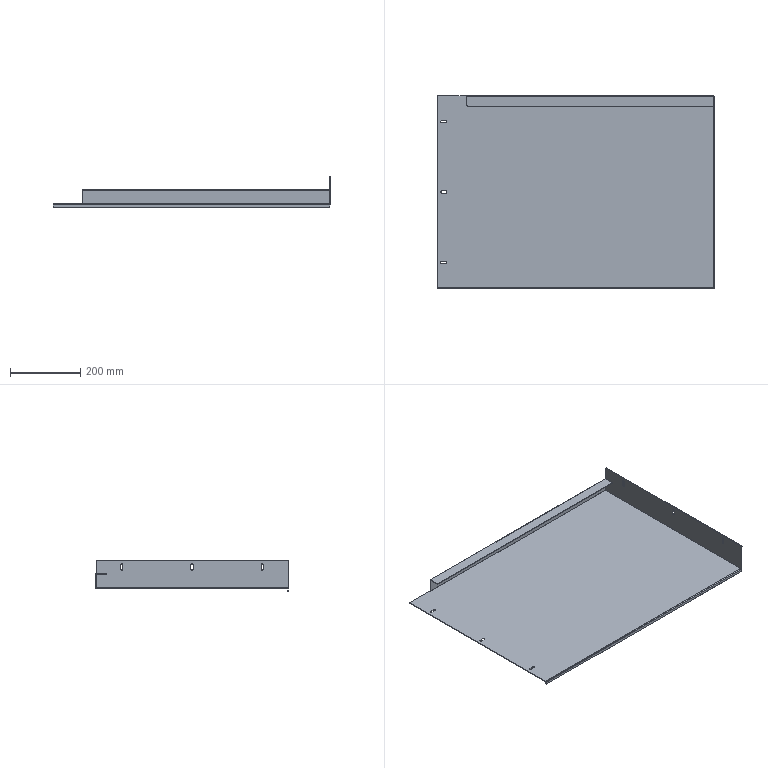Part | STEP file | 1 solid | 80 faces | box 790 x 550 x 88 mm | volume 1059109 mm3 | plane 45 | cylinder 33 | spline 2 | commonest cylinder face diameters 6 x25 0.2 x4 4.2 x4